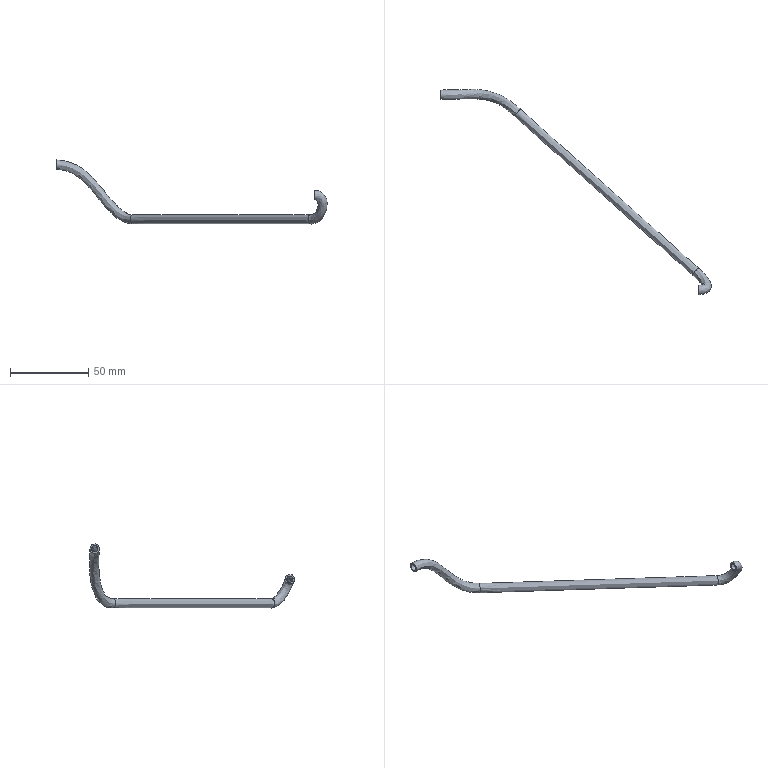Part | NX | features solid 2 | 1 solid | 8 faces | box 173.188 x 131.421 x 41.003 mm | volume 3815 mm3 | spline 6 | plane 2